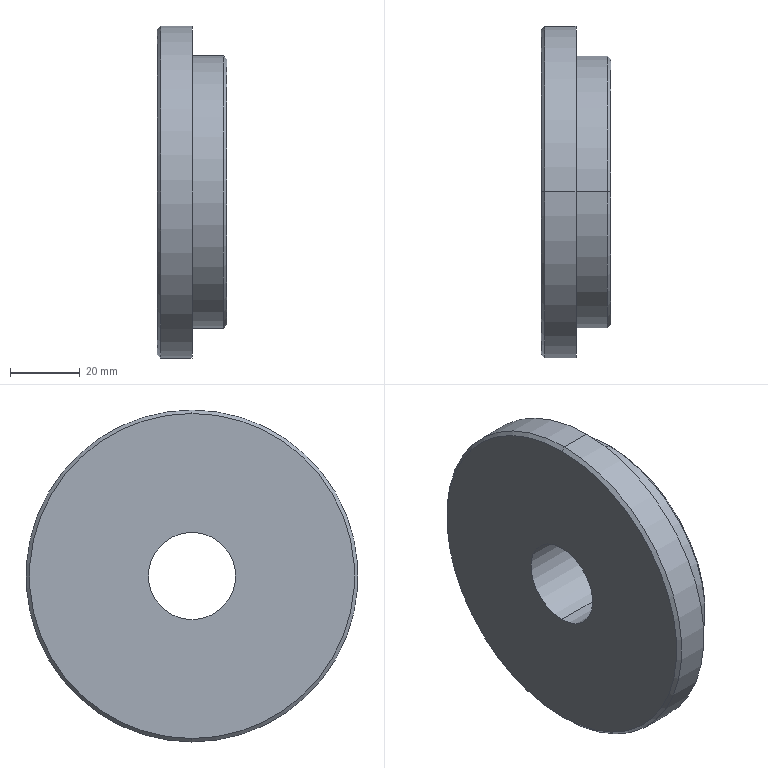Part | STEP file | Shaft end baffle | 1 solid | 13 faces | box 20 x 95 x 95 mm | volume 108579 mm3 | cylinder 6 | cone 4 | plane 3 | commonest cylinder face diameters 25 x2 78 x2 95 x2
STEP:
#1=CARTESIAN_POINT('',(0.,0.,0.));
#2=DIRECTION('',(0.,0.,1.));
#3=DIRECTION('',(1.,0.,0.));
#4=AXIS2_PLACEMENT_3D('',#1,#2,#3);
#5=CARTESIAN_POINT('',(20.,0.,38.));
#6=VERTEX_POINT('',#5);
#7=CARTESIAN_POINT('',(20.,0.,-38.));
#8=VERTEX_POINT('',#7);
#9=CARTESIAN_POINT('',(20.,0.,0.));
#10=DIRECTION('',(-1.,0.,0.));
#11=DIRECTION('',(0.,0.,1.));
#12=AXIS2_PLACEMENT_3D('',#9,#10,#11);
#13=CIRCLE('',#12,38.);
#14=CARTESIAN_POINT('',(20.,0.,0.));
#15=DIRECTION('',(-1.,0.,0.));
#16=DIRECTION('',(0.,0.,1.));
#17=AXIS2_PLACEMENT_3D('',#14,#15,#16);
#18=CONICAL_SURFACE('',#17,38.,0.7854);
#19=CARTESIAN_POINT('',(0.,0.));
#20=DIRECTION('',(1.,0.));
#21=VECTOR('',#20,1.);
#22=LINE('',#19,#21);
#23=(GEOMETRIC_REPRESENTATION_CONTEXT(2)PARAMETRIC_REPRESENTATION_CONTEXT()REPRESENTATION_CONTEXT('',''));
#24=DEFINITIONAL_REPRESENTATION('',(#22),#23);
#25=PCURVE('',#18,#24);
#26=CARTESIAN_POINT('',(20.,38.,0.));
#27=DIRECTION('',(-1.,0.,0.));
#28=DIRECTION('',(0.,0.,1.));
#29=AXIS2_PLACEMENT_3D('',#26,#27,#28);
#30=PLANE('',#29);
#31=CARTESIAN_POINT('',(0.,-38.));
#32=DIRECTION('',(1.,0.));
#33=AXIS2_PLACEMENT_2D('',#31,#32);
#34=CIRCLE('',#33,38.);
#35=(GEOMETRIC_REPRESENTATION_CONTEXT(2)PARAMETRIC_REPRESENTATION_CONTEXT()REPRESENTATION_CONTEXT('',''));
#36=DEFINITIONAL_REPRESENTATION('',(#34),#35);
#37=PCURVE('',#30,#36);
#38=SURFACE_CURVE('',#13,(#25,#37),.PCURVE_S1.);
#39=EDGE_CURVE('',#6,#8,#38,.T.);
#40=ORIENTED_EDGE('',*,*,#39,.T.);
#41=CARTESIAN_POINT('',(19.,0.,-39.));
#42=VERTEX_POINT('',#41);
#43=CARTESIAN_POINT('',(20.,0.,-38.));
#44=DIRECTION('',(-0.7071,0.,-0.7071));
#45=VECTOR('',#44,1.);
#46=LINE('',#43,#45);
#47=CARTESIAN_POINT('',(3.142,0.));
#48=DIRECTION('',(0.,1.));
#49=VECTOR('',#48,1.);
#50=LINE('',#47,#49);
#51=(GEOMETRIC_REPRESENTATION_CONTEXT(2)PARAMETRIC_REPRESENTATION_CONTEXT()REPRESENTATION_CONTEXT('',''));
#52=DEFINITIONAL_REPRESENTATION('',(#50),#51);
#53=PCURVE('',#18,#52);
#54=CARTESIAN_POINT('',(20.,0.,0.));
#55=DIRECTION('',(-1.,0.,0.));
#56=DIRECTION('',(0.,0.,1.));
#57=AXIS2_PLACEMENT_3D('',#54,#55,#56);
#58=CONICAL_SURFACE('',#57,38.,0.7854);
#59=CARTESIAN_POINT('',(3.142,0.));
#60=DIRECTION('',(0.,1.));
#61=VECTOR('',#60,1.);
#62=LINE('',#59,#61);
#63=(GEOMETRIC_REPRESENTATION_CONTEXT(2)PARAMETRIC_REPRESENTATION_CONTEXT()REPRESENTATION_CONTEXT('',''));
#64=DEFINITIONAL_REPRESENTATION('',(#62),#63);
#65=PCURVE('',#58,#64);
#66=SURFACE_CURVE('',#46,(#53,#65),.PCURVE_S1.);
#67=EDGE_CURVE('',#8,#42,#66,.T.);
#68=ORIENTED_EDGE('',*,*,#67,.T.);
#69=CARTESIAN_POINT('',(19.,0.,39.));
#70=VERTEX_POINT('',#69);
#71=CARTESIAN_POINT('',(19.,0.,0.));
#72=DIRECTION('',(-1.,0.,0.));
#73=DIRECTION('',(0.,0.,1.));
#74=AXIS2_PLACEMENT_3D('',#71,#72,#73);
#75=CIRCLE('',#74,39.);
#76=CARTESIAN_POINT('',(0.,1.));
#77=DIRECTION('',(1.,0.));
#78=VECTOR('',#77,1.);
#79=LINE('',#76,#78);
#80=(GEOMETRIC_REPRESENTATION_CONTEXT(2)PARAMETRIC_REPRESENTATION_CONTEXT()REPRESENTATION_CONTEXT('',''));
#81=DEFINITIONAL_REPRESENTATION('',(#79),#80);
#82=PCURVE('',#18,#81);
#83=CARTESIAN_POINT('',(0.,0.,0.));
#84=DIRECTION('',(-1.,0.,0.));
#85=DIRECTION('',(0.,0.,1.));
#86=AXIS2_PLACEMENT_3D('',#83,#84,#85);
#87=CYLINDRICAL_SURFACE('',#86,39.);
#88=CARTESIAN_POINT('',(0.,-19.));
#89=DIRECTION('',(1.,0.));
#90=VECTOR('',#89,1.);
#91=LINE('',#88,#90);
#92=(GEOMETRIC_REPRESENTATION_CONTEXT(2)PARAMETRIC_REPRESENTATION_CONTEXT()REPRESENTATION_CONTEXT('',''));
#93=DEFINITIONAL_REPRESENTATION('',(#91),#92);
#94=PCURVE('',#87,#93);
#95=SURFACE_CURVE('',#75,(#82,#94),.PCURVE_S1.);
#96=EDGE_CURVE('',#70,#42,#95,.T.);
#97=ORIENTED_EDGE('',*,*,#96,.F.);
#98=CARTESIAN_POINT('',(20.,0.,38.));
#99=DIRECTION('',(-0.7071,0.,0.7071));
#100=VECTOR('',#99,1.);
#101=LINE('',#98,#100);
#102=CARTESIAN_POINT('',(0.,0.));
#103=DIRECTION('',(0.,1.));
#104=VECTOR('',#103,1.);
#105=LINE('',#102,#104);
#106=(GEOMETRIC_REPRESENTATION_CONTEXT(2)PARAMETRIC_REPRESENTATION_CONTEXT()REPRESENTATION_CONTEXT('',''));
#107=DEFINITIONAL_REPRESENTATION('',(#105),#106);
#108=PCURVE('',#18,#107);
#109=CARTESIAN_POINT('',(6.283,0.));
#110=DIRECTION('',(0.,1.));
#111=VECTOR('',#110,1.);
#112=LINE('',#109,#111);
#113=(GEOMETRIC_REPRESENTATION_CONTEXT(2)PARAMETRIC_REPRESENTATION_CONTEXT()REPRESENTATION_CONTEXT('',''));
#114=DEFINITIONAL_REPRESENTATION('',(#112),#113);
#115=PCURVE('',#58,#114);
#116=SURFACE_CURVE('',#101,(#108,#115),.PCURVE_S1.);
#117=EDGE_CURVE('',#6,#70,#116,.T.);
#118=ORIENTED_EDGE('',*,*,#117,.F.);
#119=EDGE_LOOP('',(#40,#68,#97,#118));
#120=FACE_BOUND('',#119,.T.);
#121=ADVANCED_FACE('',(#120),#18,.T.);
#122=ORIENTED_EDGE('',*,*,#96,.T.);
#123=CARTESIAN_POINT('',(10.,0.,-39.));
#124=VERTEX_POINT('',#123);
#125=CARTESIAN_POINT('',(0.,0.,-39.));
#126=DIRECTION('',(-1.,0.,0.));
#127=VECTOR('',#126,1.);
#128=LINE('',#125,#127);
#129=CARTESIAN_POINT('',(3.142,0.));
#130=DIRECTION('',(0.,1.));
#131=VECTOR('',#130,1.);
#132=LINE('',#129,#131);
#133=(GEOMETRIC_REPRESENTATION_CONTEXT(2)PARAMETRIC_REPRESENTATION_CONTEXT()REPRESENTATION_CONTEXT('',''));
#134=DEFINITIONAL_REPRESENTATION('',(#132),#133);
#135=PCURVE('',#87,#134);
#136=CARTESIAN_POINT('',(0.,0.,0.));
#137=DIRECTION('',(-1.,0.,0.));
#138=DIRECTION('',(0.,0.,1.));
#139=AXIS2_PLACEMENT_3D('',#136,#137,#138);
#140=CYLINDRICAL_SURFACE('',#139,39.);
#141=CARTESIAN_POINT('',(3.142,0.));
#142=DIRECTION('',(0.,1.));
#143=VECTOR('',#142,1.);
#144=LINE('',#141,#143);
#145=(GEOMETRIC_REPRESENTATION_CONTEXT(2)PARAMETRIC_REPRESENTATION_CONTEXT()REPRESENTATION_CONTEXT('',''));
#146=DEFINITIONAL_REPRESENTATION('',(#144),#145);
#147=PCURVE('',#140,#146);
#148=SURFACE_CURVE('',#128,(#135,#147),.PCURVE_S1.);
#149=EDGE_CURVE('',#42,#124,#148,.T.);
#150=ORIENTED_EDGE('',*,*,#149,.T.);
#151=CARTESIAN_POINT('',(10.,0.,39.));
#152=VERTEX_POINT('',#151);
#153=CARTESIAN_POINT('',(10.,0.,0.));
#154=DIRECTION('',(-1.,0.,0.));
#155=DIRECTION('',(0.,0.,1.));
#156=AXIS2_PLACEMENT_3D('',#153,#154,#155);
#157=CIRCLE('',#156,39.);
#158=CARTESIAN_POINT('',(0.,-10.));
#159=DIRECTION('',(1.,0.));
#160=VECTOR('',#159,1.);
#161=LINE('',#158,#160);
#162=(GEOMETRIC_REPRESENTATION_CONTEXT(2)PARAMETRIC_REPRESENTATION_CONTEXT()REPRESENTATION_CONTEXT('',''));
#163=DEFINITIONAL_REPRESENTATION('',(#161),#162);
#164=PCURVE('',#87,#163);
#165=CARTESIAN_POINT('',(10.,47.5,0.));
#166=DIRECTION('',(-1.,0.,0.));
#167=DIRECTION('',(0.,0.,1.));
#168=AXIS2_PLACEMENT_3D('',#165,#166,#167);
#169=PLANE('',#168);
#170=CARTESIAN_POINT('',(0.,-47.5));
#171=DIRECTION('',(1.,0.));
#172=AXIS2_PLACEMENT_2D('',#170,#171);
#173=CIRCLE('',#172,39.);
#174=(GEOMETRIC_REPRESENTATION_CONTEXT(2)PARAMETRIC_REPRESENTATION_CONTEXT()REPRESENTATION_CONTEXT('',''));
#175=DEFINITIONAL_REPRESENTATION('',(#173),#174);
#176=PCURVE('',#169,#175);
#177=SURFACE_CURVE('',#157,(#164,#176),.PCURVE_S1.);
#178=EDGE_CURVE('',#152,#124,#177,.T.);
#179=ORIENTED_EDGE('',*,*,#178,.F.);
#180=CARTESIAN_POINT('',(0.,0.,39.));
#181=DIRECTION('',(-1.,0.,0.));
#182=VECTOR('',#181,1.);
#183=LINE('',#180,#182);
#184=CARTESIAN_POINT('',(0.,0.));
#185=DIRECTION('',(0.,1.));
#186=VECTOR('',#185,1.);
#187=LINE('',#184,#186);
#188=(GEOMETRIC_REPRESENTATION_CONTEXT(2)PARAMETRIC_REPRESENTATION_CONTEXT()REPRESENTATION_CONTEXT('',''));
#189=DEFINITIONAL_REPRESENTATION('',(#187),#188);
#190=PCURVE('',#87,#189);
#191=CARTESIAN_POINT('',(6.283,0.));
#192=DIRECTION('',(0.,1.));
#193=VECTOR('',#192,1.);
#194=LINE('',#191,#193);
#195=(GEOMETRIC_REPRESENTATION_CONTEXT(2)PARAMETRIC_REPRESENTATION_CONTEXT()REPRESENTATION_CONTEXT('',''));
#196=DEFINITIONAL_REPRESENTATION('',(#194),#195);
#197=PCURVE('',#140,#196);
#198=SURFACE_CURVE('',#183,(#190,#197),.PCURVE_S1.);
#199=EDGE_CURVE('',#70,#152,#198,.T.);
#200=ORIENTED_EDGE('',*,*,#199,.F.);
#201=EDGE_LOOP('',(#122,#150,#179,#200));
#202=FACE_BOUND('',#201,.T.);
#203=ADVANCED_FACE('',(#202),#87,.T.);
#204=CARTESIAN_POINT('',(10.,0.,47.5));
#205=VERTEX_POINT('',#204);
#206=CARTESIAN_POINT('',(10.,0.,-47.5));
#207=VERTEX_POINT('',#206);
#208=CARTESIAN_POINT('',(10.,0.,0.));
#209=DIRECTION('',(-1.,0.,0.));
#210=DIRECTION('',(0.,0.,1.));
#211=AXIS2_PLACEMENT_3D('',#208,#209,#210);
#212=CIRCLE('',#211,47.5);
#213=CARTESIAN_POINT('',(0.,0.,0.));
#214=DIRECTION('',(-1.,0.,0.));
#215=DIRECTION('',(0.,0.,1.));
#216=AXIS2_PLACEMENT_3D('',#213,#214,#215);
#217=CYLINDRICAL_SURFACE('',#216,47.5);
#218=CARTESIAN_POINT('',(0.,-10.));
#219=DIRECTION('',(1.,0.));
#220=VECTOR('',#219,1.);
#221=LINE('',#218,#220);
#222=(GEOMETRIC_REPRESENTATION_CONTEXT(2)PARAMETRIC_REPRESENTATION_CONTEXT()REPRESENTATION_CONTEXT('',''));
#223=DEFINITIONAL_REPRESENTATION('',(#221),#222);
#224=PCURVE('',#217,#223);
#225=CARTESIAN_POINT('',(0.,-47.5));
#226=DIRECTION('',(1.,0.));
#227=AXIS2_PLACEMENT_2D('',#225,#226);
#228=CIRCLE('',#227,47.5);
#229=(GEOMETRIC_REPRESENTATION_CONTEXT(2)PARAMETRIC_REPRESENTATION_CONTEXT()REPRESENTATION_CONTEXT('',''));
#230=DEFINITIONAL_REPRESENTATION('',(#228),#229);
#231=PCURVE('',#169,#230);
#232=SURFACE_CURVE('',#212,(#224,#231),.PCURVE_S1.);
#233=EDGE_CURVE('',#205,#207,#232,.T.);
#234=ORIENTED_EDGE('',*,*,#233,.T.);
#235=CARTESIAN_POINT('',(1.,0.,-47.5));
#236=VERTEX_POINT('',#235);
#237=CARTESIAN_POINT('',(0.,0.,-47.5));
#238=DIRECTION('',(-1.,0.,0.));
#239=VECTOR('',#238,1.);
#240=LINE('',#237,#239);
#241=CARTESIAN_POINT('',(3.142,0.));
#242=DIRECTION('',(0.,1.));
#243=VECTOR('',#242,1.);
#244=LINE('',#241,#243);
#245=(GEOMETRIC_REPRESENTATION_CONTEXT(2)PARAMETRIC_REPRESENTATION_CONTEXT()REPRESENTATION_CONTEXT('',''));
#246=DEFINITIONAL_REPRESENTATION('',(#244),#245);
#247=PCURVE('',#217,#246);
#248=CARTESIAN_POINT('',(0.,0.,0.));
#249=DIRECTION('',(-1.,0.,0.));
#250=DIRECTION('',(0.,0.,1.));
#251=AXIS2_PLACEMENT_3D('',#248,#249,#250);
#252=CYLINDRICAL_SURFACE('',#251,47.5);
#253=CARTESIAN_POINT('',(3.142,0.));
#254=DIRECTION('',(0.,1.));
#255=VECTOR('',#254,1.);
#256=LINE('',#253,#255);
#257=(GEOMETRIC_REPRESENTATION_CONTEXT(2)PARAMETRIC_REPRESENTATION_CONTEXT()REPRESENTATION_CONTEXT('',''));
#258=DEFINITIONAL_REPRESENTATION('',(#256),#257);
#259=PCURVE('',#252,#258);
#260=SURFACE_CURVE('',#240,(#247,#259),.PCURVE_S1.);
#261=EDGE_CURVE('',#207,#236,#260,.T.);
#262=ORIENTED_EDGE('',*,*,#261,.T.);
#263=CARTESIAN_POINT('',(1.,0.,47.5));
#264=VERTEX_POINT('',#263);
#265=CARTESIAN_POINT('',(1.,0.,0.));
#266=DIRECTION('',(-1.,0.,0.));
#267=DIRECTION('',(0.,0.,1.));
#268=AXIS2_PLACEMENT_3D('',#265,#266,#267);
#269=CIRCLE('',#268,47.5);
#270=CARTESIAN_POINT('',(0.,-1.));
#271=DIRECTION('',(1.,0.));
#272=VECTOR('',#271,1.);
#273=LINE('',#270,#272);
#274=(GEOMETRIC_REPRESENTATION_CONTEXT(2)PARAMETRIC_REPRESENTATION_CONTEXT()REPRESENTATION_CONTEXT('',''));
#275=DEFINITIONAL_REPRESENTATION('',(#273),#274);
#276=PCURVE('',#217,#275);
#277=CARTESIAN_POINT('',(1.,0.,0.));
#278=DIRECTION('',(1.,0.,0.));
#279=DIRECTION('',(0.,0.,-1.));
#280=AXIS2_PLACEMENT_3D('',#277,#278,#279);
#281=CONICAL_SURFACE('',#280,47.5,0.7854);
#282=CARTESIAN_POINT('',(3.142,0.));
#283=DIRECTION('',(-1.,0.));
#284=VECTOR('',#283,1.);
#285=LINE('',#282,#284);
#286=(GEOMETRIC_REPRESENTATION_CONTEXT(2)PARAMETRIC_REPRESENTATION_CONTEXT()REPRESENTATION_CONTEXT('',''));
#287=DEFINITIONAL_REPRESENTATION('',(#285),#286);
#288=PCURVE('',#281,#287);
#289=SURFACE_CURVE('',#269,(#276,#288),.PCURVE_S1.);
#290=EDGE_CURVE('',#264,#236,#289,.T.);
#291=ORIENTED_EDGE('',*,*,#290,.F.);
#292=CARTESIAN_POINT('',(0.,0.,47.5));
#293=DIRECTION('',(-1.,0.,0.));
#294=VECTOR('',#293,1.);
#295=LINE('',#292,#294);
#296=CARTESIAN_POINT('',(0.,0.));
#297=DIRECTION('',(0.,1.));
#298=VECTOR('',#297,1.);
#299=LINE('',#296,#298);
#300=(GEOMETRIC_REPRESENTATION_CONTEXT(2)PARAMETRIC_REPRESENTATION_CONTEXT()REPRESENTATION_CONTEXT('',''));
#301=DEFINITIONAL_REPRESENTATION('',(#299),#300);
#302=PCURVE('',#217,#301);
#303=CARTESIAN_POINT('',(6.283,0.));
#304=DIRECTION('',(0.,1.));
#305=VECTOR('',#304,1.);
#306=LINE('',#303,#305);
#307=(GEOMETRIC_REPRESENTATION_CONTEXT(2)PARAMETRIC_REPRESENTATION_CONTEXT()REPRESENTATION_CONTEXT('',''));
#308=DEFINITIONAL_REPRESENTATION('',(#306),#307);
#309=PCURVE('',#252,#308);
#310=SURFACE_CURVE('',#295,(#302,#309),.PCURVE_S1.);
#311=EDGE_CURVE('',#205,#264,#310,.T.);
#312=ORIENTED_EDGE('',*,*,#311,.F.);
#313=EDGE_LOOP('',(#234,#262,#291,#312));
#314=FACE_BOUND('',#313,.T.);
#315=ADVANCED_FACE('',(#314),#217,.T.);
#316=CARTESIAN_POINT('',(0.,0.,46.5));
#317=VERTEX_POINT('',#316);
#318=CARTESIAN_POINT('',(0.,0.,-46.5));
#319=VERTEX_POINT('',#318);
#320=CARTESIAN_POINT('',(0.,0.,0.));
#321=DIRECTION('',(-1.,0.,0.));
#322=DIRECTION('',(0.,0.,1.));
#323=AXIS2_PLACEMENT_3D('',#320,#321,#322);
#324=CIRCLE('',#323,46.5);
#325=CARTESIAN_POINT('',(3.142,-1.));
#326=DIRECTION('',(-1.,0.));
#327=VECTOR('',#326,1.);
#328=LINE('',#325,#327);
#329=(GEOMETRIC_REPRESENTATION_CONTEXT(2)PARAMETRIC_REPRESENTATION_CONTEXT()REPRESENTATION_CONTEXT('',''));
#330=DEFINITIONAL_REPRESENTATION('',(#328),#329);
#331=PCURVE('',#281,#330);
#332=CARTESIAN_POINT('',(0.,12.5,0.));
#333=DIRECTION('',(1.,0.,0.));
#334=DIRECTION('',(0.,0.,-1.));
#335=AXIS2_PLACEMENT_3D('',#332,#333,#334);
#336=PLANE('',#335);
#337=CARTESIAN_POINT('',(-46.5,-12.5));
#338=CARTESIAN_POINT('',(-46.5,68.04));
#339=CARTESIAN_POINT('',(23.25,27.77));
#340=CARTESIAN_POINT('',(93.,-12.5));
#341=CARTESIAN_POINT('',(23.25,-52.77));
#342=CARTESIAN_POINT('',(-46.5,-93.04));
#343=CARTESIAN_POINT('',(-46.5,-12.5));
#344=(BOUNDED_CURVE()B_SPLINE_CURVE(2,(#337,#338,#339,#340,#341,#342,#343),.UNSPECIFIED.,.T.,.F.)B_SPLINE_CURVE_WITH_KNOTS((1,2,2,2,2,1),(-2.094,0.,2.094,4.189,6.283,8.378),.UNSPECIFIED.)CURVE()GEOMETRIC_REPRESENTATION_ITEM()RATIONAL_B_SPLINE_CURVE((1.,0.5,1.,0.5,1.,0.5,1.))REPRESENTATION_ITEM(''));
#345=(GEOMETRIC_REPRESENTATION_CONTEXT(2)PARAMETRIC_REPRESENTATION_CONTEXT()REPRESENTATION_CONTEXT('',''));
#346=DEFINITIONAL_REPRESENTATION('',(#344),#345);
#347=PCURVE('',#336,#346);
#348=SURFACE_CURVE('',#324,(#331,#347),.PCURVE_S1.);
#349=EDGE_CURVE('',#317,#319,#348,.T.);
#350=ORIENTED_EDGE('',*,*,#349,.F.);
#351=CARTESIAN_POINT('',(1.,0.,47.5));
#352=DIRECTION('',(0.7071,0.,0.7071));
#353=VECTOR('',#352,1.);
#354=LINE('',#351,#353);
#355=CARTESIAN_POINT('',(3.142,0.));
#356=DIRECTION('',(0.,1.));
#357=VECTOR('',#356,1.);
#358=LINE('',#355,#357);
#359=(GEOMETRIC_REPRESENTATION_CONTEXT(2)PARAMETRIC_REPRESENTATION_CONTEXT()REPRESENTATION_CONTEXT('',''));
#360=DEFINITIONAL_REPRESENTATION('',(#358),#359);
#361=PCURVE('',#281,#360);
#362=CARTESIAN_POINT('',(1.,0.,0.));
#363=DIRECTION('',(1.,0.,0.));
#364=DIRECTION('',(0.,0.,-1.));
#365=AXIS2_PLACEMENT_3D('',#362,#363,#364);
#366=CONICAL_SURFACE('',#365,47.5,0.7854);
#367=CARTESIAN_POINT('',(3.142,0.));
#368=DIRECTION('',(0.,1.));
#369=VECTOR('',#368,1.);
#370=LINE('',#367,#369);
#371=(GEOMETRIC_REPRESENTATION_CONTEXT(2)PARAMETRIC_REPRESENTATION_CONTEXT()REPRESENTATION_CONTEXT('',''));
#372=DEFINITIONAL_REPRESENTATION('',(#370),#371);
#373=PCURVE('',#366,#372);
#374=SURFACE_CURVE('',#354,(#361,#373),.PCURVE_S1.);
#375=EDGE_CURVE('',#317,#264,#374,.T.);
#376=ORIENTED_EDGE('',*,*,#375,.T.);
#377=ORIENTED_EDGE('',*,*,#290,.T.);
#378=CARTESIAN_POINT('',(1.,0.,-47.5));
#379=DIRECTION('',(0.7071,0.,-0.7071));
#380=VECTOR('',#379,1.);
#381=LINE('',#378,#380);
#382=CARTESIAN_POINT('',(0.,0.));
#383=DIRECTION('',(0.,1.));
#384=VECTOR('',#383,1.);
#385=LINE('',#382,#384);
#386=(GEOMETRIC_REPRESENTATION_CONTEXT(2)PARAMETRIC_REPRESENTATION_CONTEXT()REPRESENTATION_CONTEXT('',''));
#387=DEFINITIONAL_REPRESENTATION('',(#385),#386);
#388=PCURVE('',#281,#387);
#389=CARTESIAN_POINT('',(6.283,0.));
#390=DIRECTION('',(0.,1.));
#391=VECTOR('',#390,1.);
#392=LINE('',#389,#391);
#393=(GEOMETRIC_REPRESENTATION_CONTEXT(2)PARAMETRIC_REPRESENTATION_CONTEXT()REPRESENTATION_CONTEXT('',''));
#394=DEFINITIONAL_REPRESENTATION('',(#392),#393);
#395=PCURVE('',#366,#394);
#396=SURFACE_CURVE('',#381,(#388,#395),.PCURVE_S1.);
#397=EDGE_CURVE('',#319,#236,#396,.T.);
#398=ORIENTED_EDGE('',*,*,#397,.F.);
#399=EDGE_LOOP('',(#350,#376,#377,#398));
#400=FACE_BOUND('',#399,.T.);
#401=ADVANCED_FACE('',(#400),#281,.T.);
#402=CARTESIAN_POINT('',(20.,0.,12.5));
#403=VERTEX_POINT('',#402);
#404=CARTESIAN_POINT('',(0.,0.,12.5));
#405=VERTEX_POINT('',#404);
#406=CARTESIAN_POINT('',(0.,0.,12.5));
#407=DIRECTION('',(-1.,0.,0.));
#408=VECTOR('',#407,1.);
#409=LINE('',#406,#408);
#410=CARTESIAN_POINT('',(0.,0.,0.));
#411=DIRECTION('',(-1.,0.,0.));
#412=DIRECTION('',(0.,0.,1.));
#413=AXIS2_PLACEMENT_3D('',#410,#411,#412);
#414=CYLINDRICAL_SURFACE('',#413,12.5);
#415=CARTESIAN_POINT('',(6.283,0.));
#416=DIRECTION('',(0.,1.));
#417=VECTOR('',#416,1.);
#418=LINE('',#415,#417);
#419=(GEOMETRIC_REPRESENTATION_CONTEXT(2)PARAMETRIC_REPRESENTATION_CONTEXT()REPRESENTATION_CONTEXT('',''));
#420=DEFINITIONAL_REPRESENTATION('',(#418),#419);
#421=PCURVE('',#414,#420);
#422=CARTESIAN_POINT('',(0.,0.,0.));
#423=DIRECTION('',(-1.,0.,0.));
#424=DIRECTION('',(0.,0.,1.));
#425=AXIS2_PLACEMENT_3D('',#422,#423,#424);
#426=CYLINDRICAL_SURFACE('',#425,12.5);
#427=CARTESIAN_POINT('',(0.,0.));
#428=DIRECTION('',(0.,1.));
#429=VECTOR('',#428,1.);
#430=LINE('',#427,#429);
#431=(GEOMETRIC_REPRESENTATION_CONTEXT(2)PARAMETRIC_REPRESENTATION_CONTEXT()REPRESENTATION_CONTEXT('',''));
#432=DEFINITIONAL_REPRESENTATION('',(#430),#431);
#433=PCURVE('',#426,#432);
#434=SURFACE_CURVE('',#409,(#421,#433),.PCURVE_S1.);
#435=EDGE_CURVE('',#403,#405,#434,.T.);
#436=ORIENTED_EDGE('',*,*,#435,.T.);
#437=CARTESIAN_POINT('',(0.,0.,-12.5));
#438=VERTEX_POINT('',#437);
#439=CARTESIAN_POINT('',(0.,0.,0.));
#440=DIRECTION('',(-1.,0.,0.));
#441=DIRECTION('',(0.,0.,1.));
#442=AXIS2_PLACEMENT_3D('',#439,#440,#441);
#443=CIRCLE('',#442,12.5);
#444=CARTESIAN_POINT('',(0.,0.));
#445=DIRECTION('',(1.,0.));
#446=VECTOR('',#445,1.);
#447=LINE('',#444,#446);
#448=(GEOMETRIC_REPRESENTATION_CONTEXT(2)PARAMETRIC_REPRESENTATION_CONTEXT()REPRESENTATION_CONTEXT('',''));
#449=DEFINITIONAL_REPRESENTATION('',(#447),#448);
#450=PCURVE('',#414,#449);
#451=CARTESIAN_POINT('',(-12.5,-12.5));
#452=CARTESIAN_POINT('',(-12.5,9.151));
#453=CARTESIAN_POINT('',(6.25,-1.675));
#454=CARTESIAN_POINT('',(25.,-12.5));
#455=CARTESIAN_POINT('',(6.25,-23.325));
#456=CARTESIAN_POINT('',(-12.5,-34.151));
#457=CARTESIAN_POINT('',(-12.5,-12.5));
#458=(BOUNDED_CURVE()B_SPLINE_CURVE(2,(#451,#452,#453,#454,#455,#456,#457),.UNSPECIFIED.,.T.,.F.)B_SPLINE_CURVE_WITH_KNOTS((1,2,2,2,2,1),(-2.094,0.,2.094,4.189,6.283,8.378),.UNSPECIFIED.)CURVE()GEOMETRIC_REPRESENTATION_ITEM()RATIONAL_B_SPLINE_CURVE((1.,0.5,1.,0.5,1.,0.5,1.))REPRESENTATION_ITEM(''));
#459=(GEOMETRIC_REPRESENTATION_CONTEXT(2)PARAMETRIC_REPRESENTATION_CONTEXT()REPRESENTATION_CONTEXT('',''));
#460=DEFINITIONAL_REPRESENTATION('',(#458),#459);
#461=PCURVE('',#336,#460);
#462=SURFACE_CURVE('',#443,(#450,#461),.PCURVE_S1.);
#463=EDGE_CURVE('',#438,#405,#462,.T.);
#464=ORIENTED_EDGE('',*,*,#463,.F.);
#465=CARTESIAN_POINT('',(20.,0.,-12.5));
#466=VERTEX_POINT('',#465);
#467=CARTESIAN_POINT('',(0.,0.,-12.5));
#468=DIRECTION('',(-1.,0.,0.));
#469=VECTOR('',#468,1.);
#470=LINE('',#467,#469);
#471=CARTESIAN_POINT('',(3.142,0.));
#472=DIRECTION('',(0.,1.));
#473=VECTOR('',#472,1.);
#474=LINE('',#471,#473);
#475=(GEOMETRIC_REPRESENTATION_CONTEXT(2)PARAMETRIC_REPRESENTATION_CONTEXT()REPRESENTATION_CONTEXT('',''));
#476=DEFINITIONAL_REPRESENTATION('',(#474),#475);
#477=PCURVE('',#414,#476);
#478=CARTESIAN_POINT('',(3.142,0.));
#479=DIRECTION('',(0.,1.));
#480=VECTOR('',#479,1.);
#481=LINE('',#478,#480);
#482=(GEOMETRIC_REPRESENTATION_CONTEXT(2)PARAMETRIC_REPRESENTATION_CONTEXT()REPRESENTATION_CONTEXT('',''));
#483=DEFINITIONAL_REPRESENTATION('',(#481),#482);
#484=PCURVE('',#426,#483);
#485=SURFACE_CURVE('',#470,(#477,#484),.PCURVE_S1.);
#486=EDGE_CURVE('',#466,#438,#485,.T.);
#487=ORIENTED_EDGE('',*,*,#486,.F.);
#488=CARTESIAN_POINT('',(20.,0.,0.));
#489=DIRECTION('',(-1.,0.,0.));
#490=DIRECTION('',(0.,0.,1.));
#491=AXIS2_PLACEMENT_3D('',#488,#489,#490);
#492=CIRCLE('',#491,12.5);
#493=CARTESIAN_POINT('',(0.,-20.));
#494=DIRECTION('',(1.,0.));
#495=VECTOR('',#494,1.);
#496=LINE('',#493,#495);
#497=(GEOMETRIC_REPRESENTATION_CONTEXT(2)PARAMETRIC_REPRESENTATION_CONTEXT()REPRESENTATION_CONTEXT('',''));
#498=DEFINITIONAL_REPRESENTATION('',(#496),#497);
#499=PCURVE('',#414,#498);
#500=CARTESIAN_POINT('',(0.,-38.));
#501=DIRECTION('',(1.,0.));
#502=AXIS2_PLACEMENT_2D('',#500,#501);
#503=CIRCLE('',#502,12.5);
#504=(GEOMETRIC_REPRESENTATION_CONTEXT(2)PARAMETRIC_REPRESENTATION_CONTEXT()REPRESENTATION_CONTEXT('',''));
#505=DEFINITIONAL_REPRESENTATION('',(#503),#504);
#506=PCURVE('',#30,#505);
#507=SURFACE_CURVE('',#492,(#499,#506),.PCURVE_S1.);
#508=EDGE_CURVE('',#466,#403,#507,.T.);
#509=ORIENTED_EDGE('',*,*,#508,.T.);
#510=EDGE_LOOP('',(#436,#464,#487,#509));
#511=FACE_BOUND('',#510,.F.);
#512=ADVANCED_FACE('',(#511),#414,.F.);
#513=CARTESIAN_POINT('',(0.,0.,0.));
#514=DIRECTION('',(-1.,0.,0.));
#515=DIRECTION('',(0.,0.,1.));
#516=AXIS2_PLACEMENT_3D('',#513,#514,#515);
#517=CIRCLE('',#516,12.5);
#518=CARTESIAN_POINT('',(0.,0.));
#519=DIRECTION('',(1.,0.));
#520=VECTOR('',#519,1.);
#521=LINE('',#518,#520);
#522=(GEOMETRIC_REPRESENTATION_CONTEXT(2)PARAMETRIC_REPRESENTATION_CONTEXT()REPRESENTATION_CONTEXT('',''));
#523=DEFINITIONAL_REPRESENTATION('',(#521),#522);
#524=PCURVE('',#426,#523);
#525=CARTESIAN_POINT('',(-12.5,-12.5));
#526=CARTESIAN_POINT('',(-12.5,9.151));
#527=CARTESIAN_POINT('',(6.25,-1.675));
#528=CARTESIAN_POINT('',(25.,-12.5));
#529=CARTESIAN_POINT('',(6.25,-23.325));
#530=CARTESIAN_POINT('',(-12.5,-34.151));
#531=CARTESIAN_POINT('',(-12.5,-12.5));
#532=(BOUNDED_CURVE()B_SPLINE_CURVE(2,(#525,#526,#527,#528,#529,#530,#531),.UNSPECIFIED.,.T.,.F.)B_SPLINE_CURVE_WITH_KNOTS((1,2,2,2,2,1),(-2.094,0.,2.094,4.189,6.283,8.378),.UNSPECIFIED.)CURVE()GEOMETRIC_REPRESENTATION_ITEM()RATIONAL_B_SPLINE_CURVE((1.,0.5,1.,0.5,1.,0.5,1.))REPRESENTATION_ITEM(''));
#533=(GEOMETRIC_REPRESENTATION_CONTEXT(2)PARAMETRIC_REPRESENTATION_CONTEXT()REPRESENTATION_CONTEXT('',''));
#534=DEFINITIONAL_REPRESENTATION('',(#532),#533);
#535=PCURVE('',#336,#534);
#536=SURFACE_CURVE('',#517,(#524,#535),.PCURVE_S1.);
#537=EDGE_CURVE('',#405,#438,#536,.T.);
#538=ORIENTED_EDGE('',*,*,#537,.F.);
#539=ORIENTED_EDGE('',*,*,#435,.F.);
#540=CARTESIAN_POINT('',(20.,0.,0.));
#541=DIRECTION('',(-1.,0.,0.));
#542=DIRECTION('',(0.,0.,1.));
#543=AXIS2_PLACEMENT_3D('',#540,#541,#542);
#544=CIRCLE('',#543,12.5);
#545=CARTESIAN_POINT('',(0.,-20.));
#546=DIRECTION('',(1.,0.));
#547=VECTOR('',#546,1.);
#548=LINE('',#545,#547);
#549=(GEOMETRIC_REPRESENTATION_CONTEXT(2)PARAMETRIC_REPRESENTATION_CONTEXT()REPRESENTATION_CONTEXT('',''));
#550=DEFINITIONAL_REPRESENTATION('',(#548),#549);
#551=PCURVE('',#426,#550);
#552=CARTESIAN_POINT('',(0.,-38.));
#553=DIRECTION('',(1.,0.));
#554=AXIS2_PLACEMENT_2D('',#552,#553);
#555=CIRCLE('',#554,12.5);
#556=(GEOMETRIC_REPRESENTATION_CONTEXT(2)PARAMETRIC_REPRESENTATION_CONTEXT()REPRESENTATION_CONTEXT('',''));
#557=DEFINITIONAL_REPRESENTATION('',(#555),#556);
#558=PCURVE('',#30,#557);
#559=SURFACE_CURVE('',#544,(#551,#558),.PCURVE_S1.);
#560=EDGE_CURVE('',#403,#466,#559,.T.);
#561=ORIENTED_EDGE('',*,*,#560,.T.);
#562=ORIENTED_EDGE('',*,*,#486,.T.);
#563=EDGE_LOOP('',(#538,#539,#561,#562));
#564=FACE_BOUND('',#563,.F.);
#565=ADVANCED_FACE('',(#564),#426,.F.);
#566=ORIENTED_EDGE('',*,*,#537,.F.);
#567=ORIENTED_EDGE('',*,*,#463,.F.);
#568=EDGE_LOOP('',(#566,#567));
#569=FACE_BOUND('',#568,.T.);
#570=CARTESIAN_POINT('',(0.,0.,0.));
#571=DIRECTION('',(-1.,0.,0.));
#572=DIRECTION('',(0.,0.,1.));
#573=AXIS2_PLACEMENT_3D('',#570,#571,#572);
#574=CIRCLE('',#573,46.5);
#575=CARTESIAN_POINT('',(-46.5,-12.5));
#576=CARTESIAN_POINT('',(-46.5,68.04));
#577=CARTESIAN_POINT('',(23.25,27.77));
#578=CARTESIAN_POINT('',(93.,-12.5));
#579=CARTESIAN_POINT('',(23.25,-52.77));
#580=CARTESIAN_POINT('',(-46.5,-93.04));
#581=CARTESIAN_POINT('',(-46.5,-12.5));
#582=(BOUNDED_CURVE()B_SPLINE_CURVE(2,(#575,#576,#577,#578,#579,#580,#581),.UNSPECIFIED.,.T.,.F.)B_SPLINE_CURVE_WITH_KNOTS((1,2,2,2,2,1),(-2.094,0.,2.094,4.189,6.283,8.378),.UNSPECIFIED.)CURVE()GEOMETRIC_REPRESENTATION_ITEM()RATIONAL_B_SPLINE_CURVE((1.,0.5,1.,0.5,1.,0.5,1.))REPRESENTATION_ITEM(''));
#583=(GEOMETRIC_REPRESENTATION_CONTEXT(2)PARAMETRIC_REPRESENTATION_CONTEXT()REPRESENTATION_CONTEXT('',''));
#584=DEFINITIONAL_REPRESENTATION('',(#582),#583);
#585=PCURVE('',#336,#584);
#586=CARTESIAN_POINT('',(9.425,-1.));
#587=DIRECTION('',(-1.,0.));
#588=VECTOR('',#587,1.);
#589=LINE('',#586,#588);
#590=(GEOMETRIC_REPRESENTATION_CONTEXT(2)PARAMETRIC_REPRESENTATION_CONTEXT()REPRESENTATION_CONTEXT('',''));
#591=DEFINITIONAL_REPRESENTATION('',(#589),#590);
#592=PCURVE('',#366,#591);
#593=SURFACE_CURVE('',#574,(#585,#592),.PCURVE_S1.);
#594=EDGE_CURVE('',#319,#317,#593,.T.);
#595=ORIENTED_EDGE('',*,*,#594,.T.);
#596=ORIENTED_EDGE('',*,*,#349,.T.);
#597=EDGE_LOOP('',(#595,#596));
#598=FACE_BOUND('',#597,.T.);
#599=ADVANCED_FACE('',(#569,#598),#336,.F.);
#600=ORIENTED_EDGE('',*,*,#375,.F.);
#601=ORIENTED_EDGE('',*,*,#594,.F.);
#602=ORIENTED_EDGE('',*,*,#397,.T.);
#603=CARTESIAN_POINT('',(1.,0.,0.));
#604=DIRECTION('',(-1.,0.,0.));
#605=DIRECTION('',(0.,0.,1.));
#606=AXIS2_PLACEMENT_3D('',#603,#604,#605);
#607=CIRCLE('',#606,47.5);
#608=CARTESIAN_POINT('',(9.425,0.));
#609=DIRECTION('',(-1.,0.));
#610=VECTOR('',#609,1.);
#611=LINE('',#608,#610);
#612=(GEOMETRIC_REPRESENTATION_CONTEXT(2)PARAMETRIC_REPRESENTATION_CONTEXT()REPRESENTATION_CONTEXT('',''));
#613=DEFINITIONAL_REPRESENTATION('',(#611),#612);
#614=PCURVE('',#366,#613);
#615=CARTESIAN_POINT('',(0.,-1.));
#616=DIRECTION('',(1.,0.));
#617=VECTOR('',#616,1.);
#618=LINE('',#615,#617);
#619=(GEOMETRIC_REPRESENTATION_CONTEXT(2)PARAMETRIC_REPRESENTATION_CONTEXT()REPRESENTATION_CONTEXT('',''));
#620=DEFINITIONAL_REPRESENTATION('',(#618),#619);
#621=PCURVE('',#252,#620);
#622=SURFACE_CURVE('',#607,(#614,#621),.PCURVE_S1.);
#623=EDGE_CURVE('',#236,#264,#622,.T.);
#624=ORIENTED_EDGE('',*,*,#623,.T.);
#625=EDGE_LOOP('',(#600,#601,#602,#624));
#626=FACE_BOUND('',#625,.T.);
#627=ADVANCED_FACE('',(#626),#366,.T.);
#628=ORIENTED_EDGE('',*,*,#261,.F.);
#629=CARTESIAN_POINT('',(10.,0.,0.));
#630=DIRECTION('',(-1.,0.,0.));
#631=DIRECTION('',(0.,0.,1.));
#632=AXIS2_PLACEMENT_3D('',#629,#630,#631);
#633=CIRCLE('',#632,47.5);
#634=CARTESIAN_POINT('',(0.,-10.));
#635=DIRECTION('',(1.,0.));
#636=VECTOR('',#635,1.);
#637=LINE('',#634,#636);
#638=(GEOMETRIC_REPRESENTATION_CONTEXT(2)PARAMETRIC_REPRESENTATION_CONTEXT()REPRESENTATION_CONTEXT('',''));
#639=DEFINITIONAL_REPRESENTATION('',(#637),#638);
#640=PCURVE('',#252,#639);
#641=CARTESIAN_POINT('',(0.,-47.5));
#642=DIRECTION('',(1.,0.));
#643=AXIS2_PLACEMENT_2D('',#641,#642);
#644=CIRCLE('',#643,47.5);
#645=(GEOMETRIC_REPRESENTATION_CONTEXT(2)PARAMETRIC_REPRESENTATION_CONTEXT()REPRESENTATION_CONTEXT('',''));
#646=DEFINITIONAL_REPRESENTATION('',(#644),#645);
#647=PCURVE('',#169,#646);
#648=SURFACE_CURVE('',#633,(#640,#647),.PCURVE_S1.);
#649=EDGE_CURVE('',#207,#205,#648,.T.);
#650=ORIENTED_EDGE('',*,*,#649,.T.);
#651=ORIENTED_EDGE('',*,*,#311,.T.);
#652=ORIENTED_EDGE('',*,*,#623,.F.);
#653=EDGE_LOOP('',(#628,#650,#651,#652));
#654=FACE_BOUND('',#653,.T.);
#655=ADVANCED_FACE('',(#654),#252,.T.);
#656=ORIENTED_EDGE('',*,*,#233,.F.);
#657=ORIENTED_EDGE('',*,*,#649,.F.);
#658=EDGE_LOOP('',(#656,#657));
#659=FACE_BOUND('',#658,.T.);
#660=ORIENTED_EDGE('',*,*,#178,.T.);
#661=CARTESIAN_POINT('',(10.,0.,0.));
#662=DIRECTION('',(-1.,0.,0.));
#663=DIRECTION('',(0.,0.,1.));
#664=AXIS2_PLACEMENT_3D('',#661,#662,#663);
#665=CIRCLE('',#664,39.);
#666=CARTESIAN_POINT('',(0.,-47.5));
#667=DIRECTION('',(1.,0.));
#668=AXIS2_PLACEMENT_2D('',#666,#667);
#669=CIRCLE('',#668,39.);
#670=(GEOMETRIC_REPRESENTATION_CONTEXT(2)PARAMETRIC_REPRESENTATION_CONTEXT()REPRESENTATION_CONTEXT('',''));
#671=DEFINITIONAL_REPRESENTATION('',(#669),#670);
#672=PCURVE('',#169,#671);
#673=CARTESIAN_POINT('',(0.,-10.));
#674=DIRECTION('',(1.,0.));
#675=VECTOR('',#674,1.);
#676=LINE('',#673,#675);
#677=(GEOMETRIC_REPRESENTATION_CONTEXT(2)PARAMETRIC_REPRESENTATION_CONTEXT()REPRESENTATION_CONTEXT('',''));
#678=DEFINITIONAL_REPRESENTATION('',(#676),#677);
#679=PCURVE('',#140,#678);
#680=SURFACE_CURVE('',#665,(#672,#679),.PCURVE_S1.);
#681=EDGE_CURVE('',#124,#152,#680,.T.);
#682=ORIENTED_EDGE('',*,*,#681,.T.);
#683=EDGE_LOOP('',(#660,#682));
#684=FACE_BOUND('',#683,.T.);
#685=ADVANCED_FACE('',(#659,#684),#169,.F.);
#686=ORIENTED_EDGE('',*,*,#149,.F.);
#687=CARTESIAN_POINT('',(19.,0.,0.));
#688=DIRECTION('',(-1.,0.,0.));
#689=DIRECTION('',(0.,0.,1.));
#690=AXIS2_PLACEMENT_3D('',#687,#688,#689);
#691=CIRCLE('',#690,39.);
#692=CARTESIAN_POINT('',(0.,-19.));
#693=DIRECTION('',(1.,0.));
#694=VECTOR('',#693,1.);
#695=LINE('',#692,#694);
#696=(GEOMETRIC_REPRESENTATION_CONTEXT(2)PARAMETRIC_REPRESENTATION_CONTEXT()REPRESENTATION_CONTEXT('',''));
#697=DEFINITIONAL_REPRESENTATION('',(#695),#696);
#698=PCURVE('',#140,#697);
#699=CARTESIAN_POINT('',(0.,1.));
#700=DIRECTION('',(1.,0.));
#701=VECTOR('',#700,1.);
#702=LINE('',#699,#701);
#703=(GEOMETRIC_REPRESENTATION_CONTEXT(2)PARAMETRIC_REPRESENTATION_CONTEXT()REPRESENTATION_CONTEXT('',''));
#704=DEFINITIONAL_REPRESENTATION('',(#702),#703);
#705=PCURVE('',#58,#704);
#706=SURFACE_CURVE('',#691,(#698,#705),.PCURVE_S1.);
#707=EDGE_CURVE('',#42,#70,#706,.T.);
#708=ORIENTED_EDGE('',*,*,#707,.T.);
#709=ORIENTED_EDGE('',*,*,#199,.T.);
#710=ORIENTED_EDGE('',*,*,#681,.F.);
#711=EDGE_LOOP('',(#686,#708,#709,#710));
#712=FACE_BOUND('',#711,.T.);
#713=ADVANCED_FACE('',(#712),#140,.T.);
#714=ORIENTED_EDGE('',*,*,#67,.F.);
#715=CARTESIAN_POINT('',(20.,0.,0.));
#716=DIRECTION('',(-1.,0.,0.));
#717=DIRECTION('',(0.,0.,1.));
#718=AXIS2_PLACEMENT_3D('',#715,#716,#717);
#719=CIRCLE('',#718,38.);
#720=CARTESIAN_POINT('',(0.,0.));
#721=DIRECTION('',(1.,0.));
#722=VECTOR('',#721,1.);
#723=LINE('',#720,#722);
#724=(GEOMETRIC_REPRESENTATION_CONTEXT(2)PARAMETRIC_REPRESENTATION_CONTEXT()REPRESENTATION_CONTEXT('',''));
#725=DEFINITIONAL_REPRESENTATION('',(#723),#724);
#726=PCURVE('',#58,#725);
#727=CARTESIAN_POINT('',(0.,-38.));
#728=DIRECTION('',(1.,0.));
#729=AXIS2_PLACEMENT_2D('',#727,#728);
#730=CIRCLE('',#729,38.);
#731=(GEOMETRIC_REPRESENTATION_CONTEXT(2)PARAMETRIC_REPRESENTATION_CONTEXT()REPRESENTATION_CONTEXT('',''));
#732=DEFINITIONAL_REPRESENTATION('',(#730),#731);
#733=PCURVE('',#30,#732);
#734=SURFACE_CURVE('',#719,(#726,#733),.PCURVE_S1.);
#735=EDGE_CURVE('',#8,#6,#734,.T.);
#736=ORIENTED_EDGE('',*,*,#735,.T.);
#737=ORIENTED_EDGE('',*,*,#117,.T.);
#738=ORIENTED_EDGE('',*,*,#707,.F.);
#739=EDGE_LOOP('',(#714,#736,#737,#738));
#740=FACE_BOUND('',#739,.T.);
#741=ADVANCED_FACE('',(#740),#58,.T.);
#742=ORIENTED_EDGE('',*,*,#39,.F.);
#743=ORIENTED_EDGE('',*,*,#735,.F.);
#744=EDGE_LOOP('',(#742,#743));
#745=FACE_BOUND('',#744,.T.);
#746=ORIENTED_EDGE('',*,*,#560,.T.);
#747=ORIENTED_EDGE('',*,*,#508,.T.);
#748=EDGE_LOOP('',(#746,#747));
#749=FACE_BOUND('',#748,.T.);
#750=ADVANCED_FACE('',(#745,#749),#30,.F.);
#751=CLOSED_SHELL('',(#121,#203,#315,#401,#512,#565,#599,#627,#655,#685,#713,#741,#750));
#752=MANIFOLD_SOLID_BREP('',#751);
#753=(LENGTH_UNIT()NAMED_UNIT(*)SI_UNIT(.MILLI.,.METRE.));
#754=UNCERTAINTY_MEASURE_WITH_UNIT(LENGTH_MEASURE(0.0000001),#753,'','');
#755=(NAMED_UNIT(*)PLANE_ANGLE_UNIT()SI_UNIT($,.RADIAN.));
#756=(NAMED_UNIT(*)SI_UNIT($,.STERADIAN.)SOLID_ANGLE_UNIT());
#757=(GEOMETRIC_REPRESENTATION_CONTEXT(3)GLOBAL_UNCERTAINTY_ASSIGNED_CONTEXT((#754))GLOBAL_UNIT_ASSIGNED_CONTEXT((#753,#755,#756))REPRESENTATION_CONTEXT('',''));
#758=ADVANCED_BREP_SHAPE_REPRESENTATION('',(#4,#752),#757);